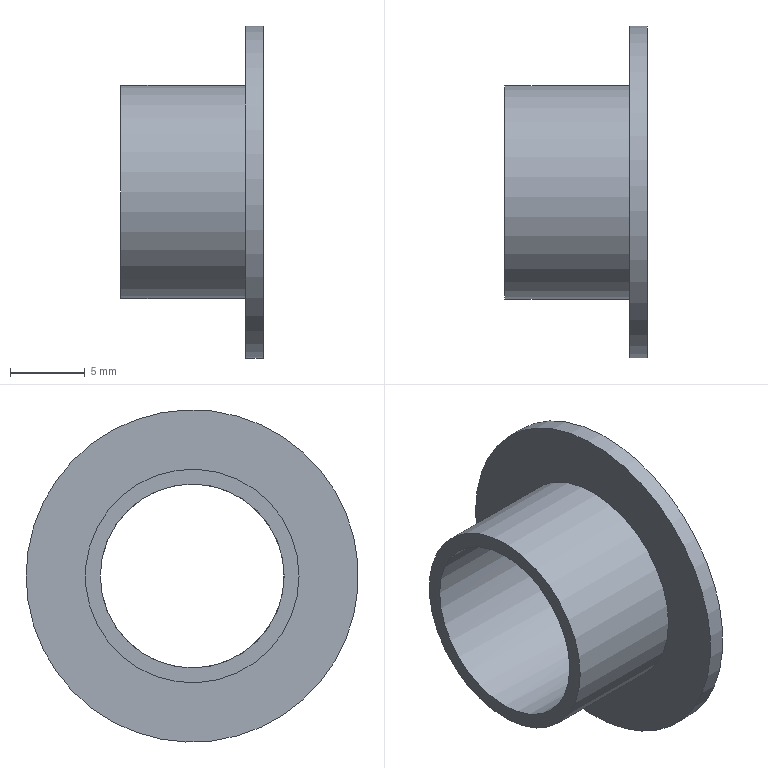Part | NX | features igus GFI bushings many(GFI-0809-06) 2 | 1 solid | 6 faces | box 9.525 x 22.225 x 22.225 mm | volume 661.266 mm3 | cylinder 3 | plane 3 | commonest cylinder face diameters 12.3 x1 14.287 x1 22.225 x1
STEP:
#1=CARTESIAN_POINT('',(-1.168,-7.144,0.));
#2=VERTEX_POINT('',#1);
#3=CARTESIAN_POINT('',(-1.168,0.,0.));
#4=DIRECTION('',(-1.,0.,0.));
#5=DIRECTION('',(0.,-1.,0.));
#6=AXIS2_PLACEMENT_3D('',#3,#4,#5);
#7=CIRCLE('',#6,7.144);
#8=EDGE_CURVE('',#2,#2,#7,.F.);
#9=ORIENTED_EDGE('',*,*,#8,.F.);
#10=EDGE_LOOP('',(#9));
#11=FACE_BOUND('',#10,.T.);
#12=CARTESIAN_POINT('',(-9.525,-7.144,0.));
#13=VERTEX_POINT('',#12);
#14=CARTESIAN_POINT('',(-9.525,0.,0.));
#15=DIRECTION('',(-1.,0.,0.));
#16=DIRECTION('',(0.,-1.,0.));
#17=AXIS2_PLACEMENT_3D('',#14,#15,#16);
#18=CIRCLE('',#17,7.144);
#19=EDGE_CURVE('',#13,#13,#18,.F.);
#20=ORIENTED_EDGE('',*,*,#19,.T.);
#21=EDGE_LOOP('',(#20));
#22=FACE_BOUND('',#21,.T.);
#23=CARTESIAN_POINT('',(0.,0.,0.));
#24=DIRECTION('',(1.,0.,0.));
#25=DIRECTION('',(0.,1.,0.));
#26=AXIS2_PLACEMENT_3D('',#23,#24,#25);
#27=CYLINDRICAL_SURFACE('',#26,7.144);
#28=ADVANCED_FACE('',(#11,#22),#27,.T.);
#29=ORIENTED_EDGE('',*,*,#19,.F.);
#30=EDGE_LOOP('',(#29));
#31=FACE_BOUND('',#30,.T.);
#32=CARTESIAN_POINT('',(-9.525,-6.15,0.));
#33=VERTEX_POINT('',#32);
#34=CARTESIAN_POINT('',(-9.525,0.,0.));
#35=DIRECTION('',(-1.,0.,0.));
#36=DIRECTION('',(0.,-1.,0.));
#37=AXIS2_PLACEMENT_3D('',#34,#35,#36);
#38=CIRCLE('',#37,6.15);
#39=EDGE_CURVE('',#33,#33,#38,.F.);
#40=ORIENTED_EDGE('',*,*,#39,.T.);
#41=EDGE_LOOP('',(#40));
#42=FACE_BOUND('',#41,.T.);
#43=CARTESIAN_POINT('',(-9.525,6.35,0.));
#44=DIRECTION('',(-1.,0.,0.));
#45=DIRECTION('',(0.,-1.,0.));
#46=AXIS2_PLACEMENT_3D('',#43,#44,#45);
#47=PLANE('',#46);
#48=ADVANCED_FACE('',(#31,#42),#47,.T.);
#49=ORIENTED_EDGE('',*,*,#8,.T.);
#50=EDGE_LOOP('',(#49));
#51=FACE_BOUND('',#50,.T.);
#52=CARTESIAN_POINT('',(-1.168,11.113,0.));
#53=VERTEX_POINT('',#52);
#54=CARTESIAN_POINT('',(-1.168,0.,0.));
#55=DIRECTION('',(1.,0.,0.));
#56=DIRECTION('',(0.,1.,0.));
#57=AXIS2_PLACEMENT_3D('',#54,#55,#56);
#58=CIRCLE('',#57,11.113);
#59=EDGE_CURVE('',#53,#53,#58,.T.);
#60=ORIENTED_EDGE('',*,*,#59,.F.);
#61=EDGE_LOOP('',(#60));
#62=FACE_BOUND('',#61,.T.);
#63=CARTESIAN_POINT('',(-1.168,7.541,0.));
#64=DIRECTION('',(-1.,0.,0.));
#65=DIRECTION('',(0.,-1.,0.));
#66=AXIS2_PLACEMENT_3D('',#63,#64,#65);
#67=PLANE('',#66);
#68=ADVANCED_FACE('',(#51,#62),#67,.T.);
#69=ORIENTED_EDGE('',*,*,#59,.T.);
#70=EDGE_LOOP('',(#69));
#71=FACE_BOUND('',#70,.T.);
#72=CARTESIAN_POINT('',(0.,11.113,0.));
#73=VERTEX_POINT('',#72);
#74=CARTESIAN_POINT('',(0.,0.,0.));
#75=DIRECTION('',(1.,0.,0.));
#76=DIRECTION('',(0.,1.,0.));
#77=AXIS2_PLACEMENT_3D('',#74,#75,#76);
#78=CIRCLE('',#77,11.113);
#79=EDGE_CURVE('',#73,#73,#78,.T.);
#80=ORIENTED_EDGE('',*,*,#79,.F.);
#81=EDGE_LOOP('',(#80));
#82=FACE_BOUND('',#81,.T.);
#83=CARTESIAN_POINT('',(0.,0.,0.));
#84=DIRECTION('',(1.,0.,0.));
#85=DIRECTION('',(0.,1.,0.));
#86=AXIS2_PLACEMENT_3D('',#83,#84,#85);
#87=CYLINDRICAL_SURFACE('',#86,11.113);
#88=ADVANCED_FACE('',(#71,#82),#87,.T.);
#89=ORIENTED_EDGE('',*,*,#79,.T.);
#90=EDGE_LOOP('',(#89));
#91=FACE_BOUND('',#90,.T.);
#92=CARTESIAN_POINT('',(0.,6.15,0.));
#93=VERTEX_POINT('',#92);
#94=CARTESIAN_POINT('',(0.,0.,0.));
#95=DIRECTION('',(1.,0.,0.));
#96=DIRECTION('',(0.,1.,0.));
#97=AXIS2_PLACEMENT_3D('',#94,#95,#96);
#98=CIRCLE('',#97,6.15);
#99=EDGE_CURVE('',#93,#93,#98,.T.);
#100=ORIENTED_EDGE('',*,*,#99,.F.);
#101=EDGE_LOOP('',(#100));
#102=FACE_BOUND('',#101,.T.);
#103=CARTESIAN_POINT('',(0.,6.35,0.));
#104=DIRECTION('',(1.,0.,0.));
#105=DIRECTION('',(0.,1.,0.));
#106=AXIS2_PLACEMENT_3D('',#103,#104,#105);
#107=PLANE('',#106);
#108=ADVANCED_FACE('',(#91,#102),#107,.T.);
#109=ORIENTED_EDGE('',*,*,#99,.T.);
#110=EDGE_LOOP('',(#109));
#111=FACE_BOUND('',#110,.T.);
#112=ORIENTED_EDGE('',*,*,#39,.F.);
#113=EDGE_LOOP('',(#112));
#114=FACE_BOUND('',#113,.T.);
#115=CARTESIAN_POINT('',(0.,0.,0.));
#116=DIRECTION('',(1.,0.,0.));
#117=DIRECTION('',(0.,1.,0.));
#118=AXIS2_PLACEMENT_3D('',#115,#116,#117);
#119=CYLINDRICAL_SURFACE('',#118,6.15);
#120=ADVANCED_FACE('',(#111,#114),#119,.F.);
#121=CLOSED_SHELL('',(#28,#48,#68,#88,#108,#120));
#122=MANIFOLD_SOLID_BREP('',#121);
#123=(LENGTH_UNIT()NAMED_UNIT(*)SI_UNIT(.MILLI.,.METRE.));
#124=UNCERTAINTY_MEASURE_WITH_UNIT(LENGTH_MEASURE(0.00001),#123,'','');
#125=(NAMED_UNIT(*)PLANE_ANGLE_UNIT()SI_UNIT($,.RADIAN.));
#126=(NAMED_UNIT(*)SI_UNIT($,.STERADIAN.)SOLID_ANGLE_UNIT());
#127=(GEOMETRIC_REPRESENTATION_CONTEXT(3)GLOBAL_UNCERTAINTY_ASSIGNED_CONTEXT((#124))GLOBAL_UNIT_ASSIGNED_CONTEXT((#123,#125,#126))REPRESENTATION_CONTEXT('',''));
#128=ADVANCED_BREP_SHAPE_REPRESENTATION('',(#122),#127);